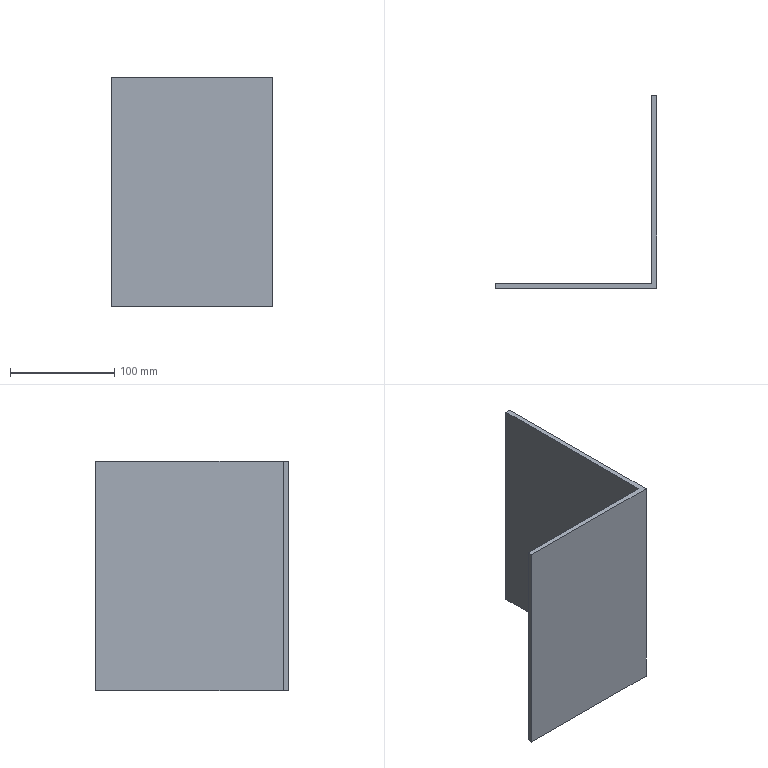Part | SolidWorks | features Extrusion 1 | 1 solid | 8 faces | box 155 x 185 x 220 mm | volume 368500 mm3 | plane 8
STEP:
#1=CARTESIAN_POINT('',(-155.,5.,110.));
#2=VERTEX_POINT('',#1);
#3=CARTESIAN_POINT('',(-155.,0.,110.));
#4=VERTEX_POINT('',#3);
#5=CARTESIAN_POINT('',(-155.,5.,110.));
#6=DIRECTION('',(0.,-1.,0.));
#7=VECTOR('',#6,1000.);
#8=LINE('',#5,#7);
#9=EDGE_CURVE('',#2,#4,#8,.T.);
#10=ORIENTED_EDGE('',*,*,#9,.F.);
#11=CARTESIAN_POINT('',(-155.,5.,-110.));
#12=VERTEX_POINT('',#11);
#13=CARTESIAN_POINT('',(-155.,5.,-110.));
#14=DIRECTION('',(0.,0.,1.));
#15=VECTOR('',#14,1000.);
#16=LINE('',#13,#15);
#17=EDGE_CURVE('',#12,#2,#16,.T.);
#18=ORIENTED_EDGE('',*,*,#17,.F.);
#19=CARTESIAN_POINT('',(-155.,0.,-110.));
#20=VERTEX_POINT('',#19);
#21=CARTESIAN_POINT('',(-155.,5.,-110.));
#22=DIRECTION('',(0.,-1.,0.));
#23=VECTOR('',#22,1000.);
#24=LINE('',#21,#23);
#25=EDGE_CURVE('',#12,#20,#24,.T.);
#26=ORIENTED_EDGE('',*,*,#25,.T.);
#27=CARTESIAN_POINT('',(-155.,0.,-110.));
#28=DIRECTION('',(0.,0.,1.));
#29=VECTOR('',#28,1000.);
#30=LINE('',#27,#29);
#31=EDGE_CURVE('',#20,#4,#30,.T.);
#32=ORIENTED_EDGE('',*,*,#31,.T.);
#33=EDGE_LOOP('',(#10,#18,#26,#32));
#34=FACE_OUTER_BOUND('',#33,.T.);
#35=CARTESIAN_POINT('',(-155.,5.,-110.));
#36=DIRECTION('',(-1.,0.,0.));
#37=DIRECTION('',(0.,0.,1.));
#38=AXIS2_PLACEMENT_3D('',#35,#36,#37);
#39=PLANE('',#38);
#40=ADVANCED_FACE('',(#34),#39,.T.);
#41=CARTESIAN_POINT('',(-5.,5.,110.));
#42=VERTEX_POINT('',#41);
#43=CARTESIAN_POINT('',(-5.,5.,110.));
#44=DIRECTION('',(-1.,0.,0.));
#45=VECTOR('',#44,1000.);
#46=LINE('',#43,#45);
#47=EDGE_CURVE('',#42,#2,#46,.T.);
#48=ORIENTED_EDGE('',*,*,#47,.F.);
#49=CARTESIAN_POINT('',(-5.,5.,-110.));
#50=VERTEX_POINT('',#49);
#51=CARTESIAN_POINT('',(-5.,5.,-110.));
#52=DIRECTION('',(0.,0.,1.));
#53=VECTOR('',#52,1000.);
#54=LINE('',#51,#53);
#55=EDGE_CURVE('',#50,#42,#54,.T.);
#56=ORIENTED_EDGE('',*,*,#55,.F.);
#57=CARTESIAN_POINT('',(-5.,5.,-110.));
#58=DIRECTION('',(-1.,0.,0.));
#59=VECTOR('',#58,1000.);
#60=LINE('',#57,#59);
#61=EDGE_CURVE('',#50,#12,#60,.T.);
#62=ORIENTED_EDGE('',*,*,#61,.T.);
#63=ORIENTED_EDGE('',*,*,#17,.T.);
#64=EDGE_LOOP('',(#48,#56,#62,#63));
#65=FACE_OUTER_BOUND('',#64,.T.);
#66=CARTESIAN_POINT('',(-5.,5.,-110.));
#67=DIRECTION('',(0.,1.,0.));
#68=DIRECTION('',(0.,0.,1.));
#69=AXIS2_PLACEMENT_3D('',#66,#67,#68);
#70=PLANE('',#69);
#71=ADVANCED_FACE('',(#65),#70,.T.);
#72=CARTESIAN_POINT('',(-5.,185.,110.));
#73=VERTEX_POINT('',#72);
#74=CARTESIAN_POINT('',(-5.,185.,110.));
#75=DIRECTION('',(0.,-1.,0.));
#76=VECTOR('',#75,1000.);
#77=LINE('',#74,#76);
#78=EDGE_CURVE('',#73,#42,#77,.T.);
#79=ORIENTED_EDGE('',*,*,#78,.F.);
#80=CARTESIAN_POINT('',(-5.,185.,-110.));
#81=VERTEX_POINT('',#80);
#82=CARTESIAN_POINT('',(-5.,185.,-110.));
#83=DIRECTION('',(0.,0.,1.));
#84=VECTOR('',#83,1000.);
#85=LINE('',#82,#84);
#86=EDGE_CURVE('',#81,#73,#85,.T.);
#87=ORIENTED_EDGE('',*,*,#86,.F.);
#88=CARTESIAN_POINT('',(-5.,185.,-110.));
#89=DIRECTION('',(0.,-1.,0.));
#90=VECTOR('',#89,1000.);
#91=LINE('',#88,#90);
#92=EDGE_CURVE('',#81,#50,#91,.T.);
#93=ORIENTED_EDGE('',*,*,#92,.T.);
#94=ORIENTED_EDGE('',*,*,#55,.T.);
#95=EDGE_LOOP('',(#79,#87,#93,#94));
#96=FACE_OUTER_BOUND('',#95,.T.);
#97=CARTESIAN_POINT('',(-5.,185.,-110.));
#98=DIRECTION('',(-1.,0.,0.));
#99=DIRECTION('',(0.,0.,1.));
#100=AXIS2_PLACEMENT_3D('',#97,#98,#99);
#101=PLANE('',#100);
#102=ADVANCED_FACE('',(#96),#101,.T.);
#103=CARTESIAN_POINT('',(0.,185.,110.));
#104=VERTEX_POINT('',#103);
#105=CARTESIAN_POINT('',(0.,185.,110.));
#106=DIRECTION('',(-1.,0.,0.));
#107=VECTOR('',#106,1000.);
#108=LINE('',#105,#107);
#109=EDGE_CURVE('',#104,#73,#108,.T.);
#110=ORIENTED_EDGE('',*,*,#109,.F.);
#111=CARTESIAN_POINT('',(0.,185.,-110.));
#112=VERTEX_POINT('',#111);
#113=CARTESIAN_POINT('',(0.,185.,-110.));
#114=DIRECTION('',(0.,0.,1.));
#115=VECTOR('',#114,1000.);
#116=LINE('',#113,#115);
#117=EDGE_CURVE('',#112,#104,#116,.T.);
#118=ORIENTED_EDGE('',*,*,#117,.F.);
#119=CARTESIAN_POINT('',(0.,185.,-110.));
#120=DIRECTION('',(-1.,0.,0.));
#121=VECTOR('',#120,1000.);
#122=LINE('',#119,#121);
#123=EDGE_CURVE('',#112,#81,#122,.T.);
#124=ORIENTED_EDGE('',*,*,#123,.T.);
#125=ORIENTED_EDGE('',*,*,#86,.T.);
#126=EDGE_LOOP('',(#110,#118,#124,#125));
#127=FACE_OUTER_BOUND('',#126,.T.);
#128=CARTESIAN_POINT('',(0.,185.,-110.));
#129=DIRECTION('',(0.,1.,0.));
#130=DIRECTION('',(0.,0.,1.));
#131=AXIS2_PLACEMENT_3D('',#128,#129,#130);
#132=PLANE('',#131);
#133=ADVANCED_FACE('',(#127),#132,.T.);
#134=CARTESIAN_POINT('',(0.,0.,110.));
#135=VERTEX_POINT('',#134);
#136=CARTESIAN_POINT('',(0.,0.,110.));
#137=DIRECTION('',(0.,1.,0.));
#138=VECTOR('',#137,1000.);
#139=LINE('',#136,#138);
#140=EDGE_CURVE('',#135,#104,#139,.T.);
#141=ORIENTED_EDGE('',*,*,#140,.F.);
#142=CARTESIAN_POINT('',(0.,0.,-110.));
#143=VERTEX_POINT('',#142);
#144=CARTESIAN_POINT('',(0.,0.,-110.));
#145=DIRECTION('',(0.,0.,1.));
#146=VECTOR('',#145,1000.);
#147=LINE('',#144,#146);
#148=EDGE_CURVE('',#143,#135,#147,.T.);
#149=ORIENTED_EDGE('',*,*,#148,.F.);
#150=CARTESIAN_POINT('',(0.,0.,-110.));
#151=DIRECTION('',(0.,1.,0.));
#152=VECTOR('',#151,1000.);
#153=LINE('',#150,#152);
#154=EDGE_CURVE('',#143,#112,#153,.T.);
#155=ORIENTED_EDGE('',*,*,#154,.T.);
#156=ORIENTED_EDGE('',*,*,#117,.T.);
#157=EDGE_LOOP('',(#141,#149,#155,#156));
#158=FACE_OUTER_BOUND('',#157,.T.);
#159=CARTESIAN_POINT('',(0.,0.,-110.));
#160=DIRECTION('',(1.,0.,0.));
#161=DIRECTION('',(0.,0.,-1.));
#162=AXIS2_PLACEMENT_3D('',#159,#160,#161);
#163=PLANE('',#162);
#164=ADVANCED_FACE('',(#158),#163,.T.);
#165=CARTESIAN_POINT('',(-155.,0.,110.));
#166=DIRECTION('',(1.,0.,0.));
#167=VECTOR('',#166,1000.);
#168=LINE('',#165,#167);
#169=EDGE_CURVE('',#4,#135,#168,.T.);
#170=ORIENTED_EDGE('',*,*,#169,.F.);
#171=ORIENTED_EDGE('',*,*,#31,.F.);
#172=CARTESIAN_POINT('',(-155.,0.,-110.));
#173=DIRECTION('',(1.,0.,0.));
#174=VECTOR('',#173,1000.);
#175=LINE('',#172,#174);
#176=EDGE_CURVE('',#20,#143,#175,.T.);
#177=ORIENTED_EDGE('',*,*,#176,.T.);
#178=ORIENTED_EDGE('',*,*,#148,.T.);
#179=EDGE_LOOP('',(#170,#171,#177,#178));
#180=FACE_OUTER_BOUND('',#179,.T.);
#181=CARTESIAN_POINT('',(-155.,0.,-110.));
#182=DIRECTION('',(0.,-1.,0.));
#183=DIRECTION('',(0.,0.,-1.));
#184=AXIS2_PLACEMENT_3D('',#181,#182,#183);
#185=PLANE('',#184);
#186=ADVANCED_FACE('',(#180),#185,.T.);
#187=ORIENTED_EDGE('',*,*,#25,.F.);
#188=ORIENTED_EDGE('',*,*,#61,.F.);
#189=ORIENTED_EDGE('',*,*,#92,.F.);
#190=ORIENTED_EDGE('',*,*,#123,.F.);
#191=ORIENTED_EDGE('',*,*,#154,.F.);
#192=ORIENTED_EDGE('',*,*,#176,.F.);
#193=EDGE_LOOP('',(#187,#188,#189,#190,#191,#192));
#194=FACE_OUTER_BOUND('',#193,.T.);
#195=CARTESIAN_POINT('',(0.,0.,-110.));
#196=DIRECTION('',(0.,0.,1.));
#197=DIRECTION('',(1.,0.,0.));
#198=AXIS2_PLACEMENT_3D('',#195,#196,#197);
#199=PLANE('',#198);
#200=ADVANCED_FACE('',(#194),#199,.F.);
#201=ORIENTED_EDGE('',*,*,#9,.T.);
#202=ORIENTED_EDGE('',*,*,#169,.T.);
#203=ORIENTED_EDGE('',*,*,#140,.T.);
#204=ORIENTED_EDGE('',*,*,#109,.T.);
#205=ORIENTED_EDGE('',*,*,#78,.T.);
#206=ORIENTED_EDGE('',*,*,#47,.T.);
#207=EDGE_LOOP('',(#201,#202,#203,#204,#205,#206));
#208=FACE_OUTER_BOUND('',#207,.T.);
#209=CARTESIAN_POINT('',(0.,0.,110.));
#210=DIRECTION('',(0.,0.,1.));
#211=DIRECTION('',(1.,0.,0.));
#212=AXIS2_PLACEMENT_3D('',#209,#210,#211);
#213=PLANE('',#212);
#214=ADVANCED_FACE('',(#208),#213,.T.);
#215=CLOSED_SHELL('',(#40,#71,#102,#133,#164,#186,#200,#214));
#216=MANIFOLD_SOLID_BREP('',#215);
#217=CARTESIAN_POINT('',(0.,0.,0.));
#218=DIRECTION('',(0.,0.,1.));
#219=DIRECTION('',(1.,0.,0.));
#220=AXIS2_PLACEMENT_3D('',#217,#218,#219);
#221=(LENGTH_UNIT()NAMED_UNIT(*)SI_UNIT(.MILLI.,.METRE.));
#222=UNCERTAINTY_MEASURE_WITH_UNIT(LENGTH_MEASURE(0.00001),#221,'','');
#223=(NAMED_UNIT(*)PLANE_ANGLE_UNIT()SI_UNIT($,.RADIAN.));
#224=(NAMED_UNIT(*)SI_UNIT($,.STERADIAN.)SOLID_ANGLE_UNIT());
#225=(GEOMETRIC_REPRESENTATION_CONTEXT(3)GLOBAL_UNCERTAINTY_ASSIGNED_CONTEXT((#222))GLOBAL_UNIT_ASSIGNED_CONTEXT((#221,#223,#224))REPRESENTATION_CONTEXT('',''));
#226=ADVANCED_BREP_SHAPE_REPRESENTATION('',(#216,#220),#225);